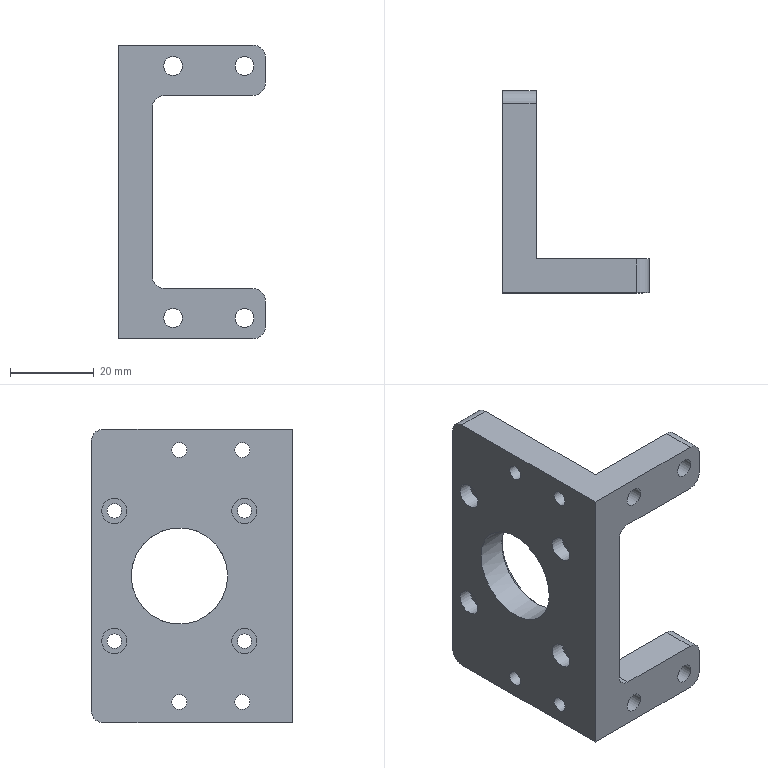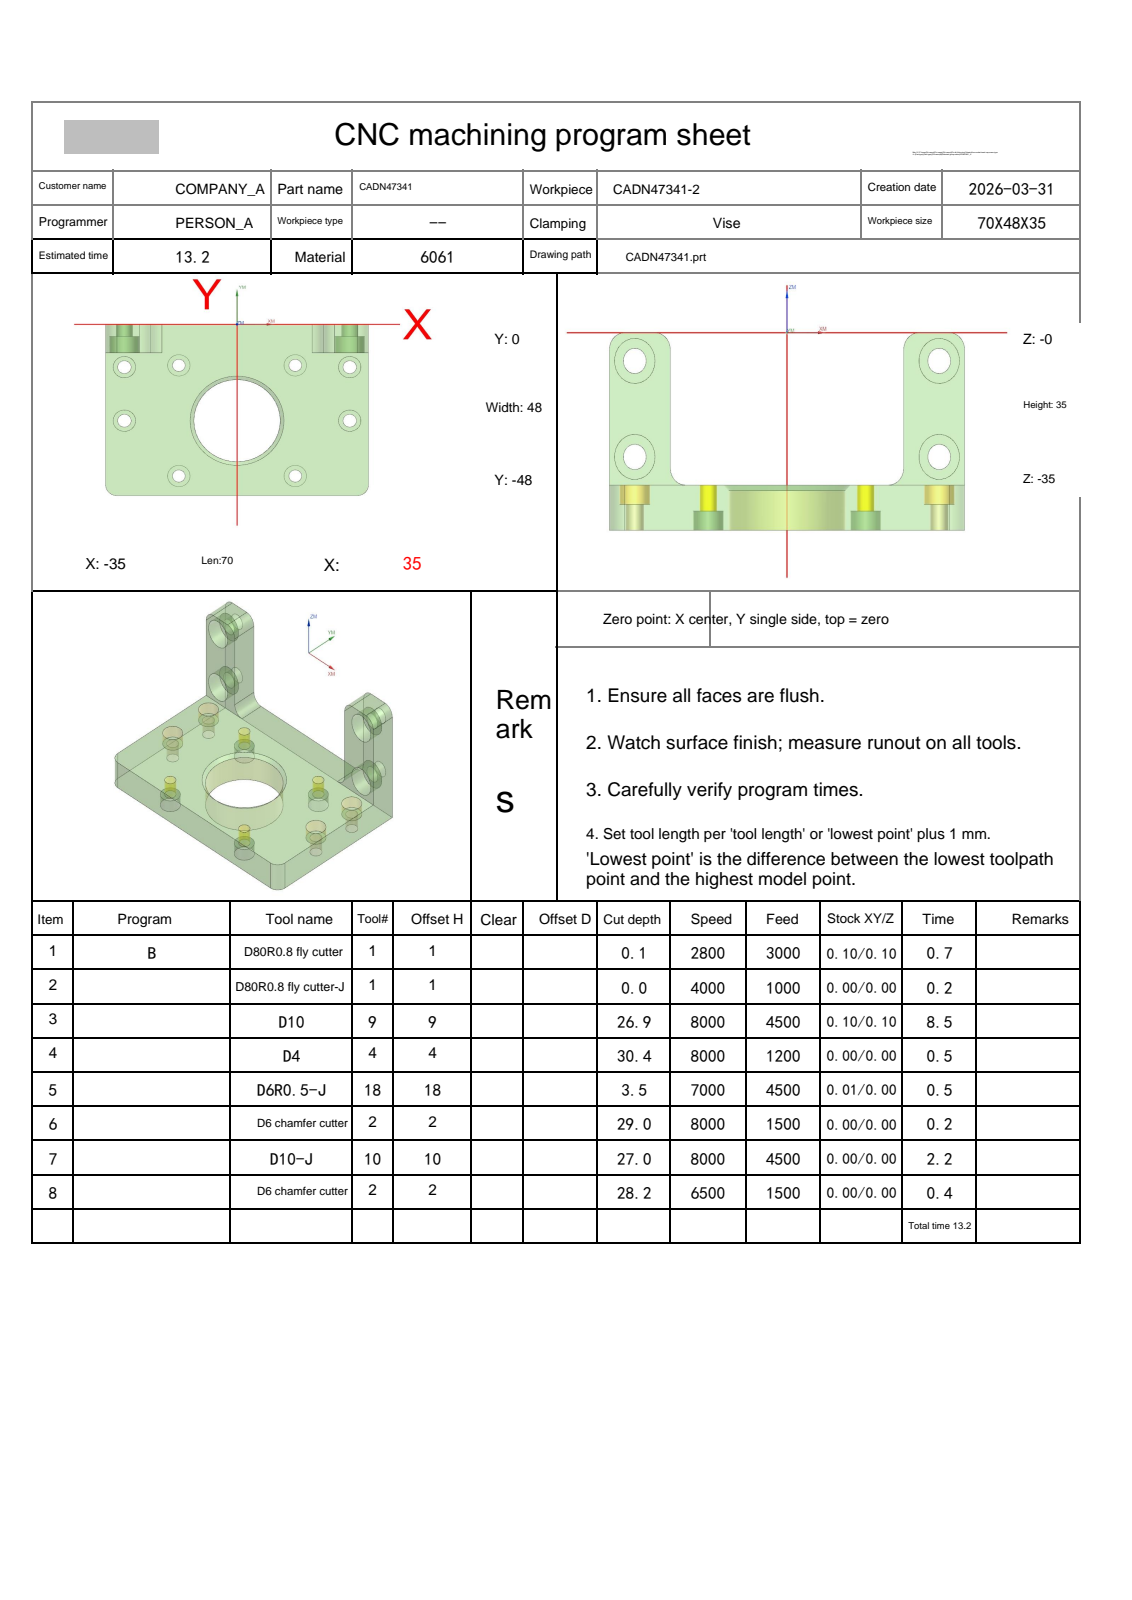NC program | NX | posted by the shop | part box 35 x 48 x 70 mm
Lines 9806 to 11022 of 13995:
N7 T10 M06
(D10-J  D=10. R=0. H=10 ce=0.40 di=0.00)
G00 G90 G54 X2. Y-55. M03 S7000
G43 H10 Z14.5
M08
Z-25.5
G01 Z-27. F1500.
Y-51.
G03 X0.0 Y-49. I-2. J0.0
G01 X-32.001
G02 X-36. Y-45. I.001 J4.
G01 Y-14.397
G02 X-35.003 Y-13.4 I1. J-.003
G01 X-14.6
Y.003
G02 X-13.603 Y1. I1. J-.003
G01 X13.603
G02 X14.6 Y.003 I-.003 J-1.
G01 Y-13.4
X35.003
G02 X36. Y-14.397 I-.003 J-1.
G01 Y-45.
G02 X32. Y-49. I-4. J0.0
G01 X-2.086
G02 X-2.793 Y-48.707 I.001 J1.
G01 X-7.207 Y-44.293
G03 X-7.914 Y-44. I-.707 J-.707
G01 X-30.003
G02 X-31. Y-43.003 I.003 J1.
G01 Y-19.397
G02 X-30.003 Y-18.4 I1. J-.003
G01 X-14.6
G03 X-9.6 Y-13.4 I0.0 J5.
G01 Y-4.997
G02 X-8.603 Y-4. I1. J-.003
G01 X8.603
G02 X9.6 Y-4.997 I-.003 J-1.
G01 Y-13.4
G03 X14.6 Y-18.4 I5. J0.0
G01 X30.003
G02 X31. Y-19.397 I-.003 J-1.
G01 Y-43.003
G02 X30.003 Y-44. I-1. J.003
G01 X-2.086
G02 X-2.793 Y-43.707 I0.0 J1.
G01 X-7.207 Y-39.293
G03 X-7.914 Y-39. I-.707 J-.707
G01 X-25.003
G02 X-26. Y-38.003 I.003 J1.
G01 Y-24.397
G02 X-25.003 Y-23.4 I1. J-.003
G01 X-14.6
G03 X-4.6 Y-13.4 I0.0 J10.
G01 Y-9.997
G02 X-3.603 Y-9. I1. J-.003
G01 X3.603
G02 X4.6 Y-9.997 I-.003 J-1.
G01 Y-13.4
G03 X14.6 Y-23.4 I10. J0.0
G01 X25.003
G02 X26. Y-24.397 I-.003 J-1.
G01 Y-38.003
G02 X25.003 Y-39. I-1. J.003
G01 X-2.086
G02 X-2.793 Y-38.707 I0.0 J1.
G01 X-7.207 Y-34.293
G03 X-7.914 Y-34. I-.707 J-.707
G01 X-20.003
G02 X-21. Y-33.003 I.003 J1.
G01 Y-29.397
G02 X-20.003 Y-28.4 I1. J-.003
G01 X-14.6
G03 X-.911 Y-19.533 I0.0 J15.
G02 X0.0 Y-18.945 I.911 J-.412
X.911 Y-19.533 I0.0 J-1.
G03 X14.6 Y-28.4 I13.689 J6.133
G01 X20.003
G02 X21. Y-29.397 I-.003 J-1.
G01 Y-33.003
G02 X20.003 Y-34. I-1. J.003
G01 X-1.511
G02 X-2.211 Y-33.3 I0.0 J.7
X-2.171 Y-33.067 I.7 J0.0
G01 X-1.072 Y-29.948
G03 X-.888 Y-28.876 I-3.044 J1.073
X-.923 Y-28.403 I-3.227 J0.0
G01 X-.931 Y-28.3
G02 X-.719 Y-27.798 I.7 J0.0
G03 X-.492 Y-27.576 I-13.881 J14.398
G02 X0.0 Y-27.374 I.492 J-.498
X.492 Y-27.576 I0.0 J-.7
G03 X.719 Y-27.798 I14.108 J14.176
G02 X.931 Y-28.3 I-.488 J-.502
X.233 Y-29. I-.7 J0.0
G01 X-.233
G02 X-.68 Y-28.837 I.003 J.7
X-.931 Y-28.3 I.449 J.537
X-.826 Y-27.931 I.7 J0.0
G03 X-.526 Y-26.878 I-1.7 J1.053
X-1.473 Y-25.178 I-2. J0.0
G01 Z-25.5
G00 Z14.5
G00 G90 X-13.5 Y-14.7 M03 S8000
Z14.5
Z-12.
G01 Z-13.5 F1000.
G41 D10
Y-14.5
G03 X-15. Y-13. I-1.5 J0.0
G01 X-40.
G03 X-41.5 Y-14.5 I0.0 J-1.5
G01 G40 Y-14.7
Z-12.
G00 X-13.5
Z-25.5
G01 Z-27.
G41 D10
Y-14.5
G03 X-15. Y-13. I-1.5 J0.0
G01 X-40.003
G03 X-41.5 Y-14.405 I0.0 J-1.5
G01 G40 X-41.513 Y-14.605
Z-25.5
G00 Z3.
X41.5 Y-14.7
Z-12.
G01 Z-13.5
G41 D10
Y-14.5
G03 X40. Y-13. I-1.5 J0.0
G01 X15.
G03 X13.5 Y-14.5 I0.0 J-1.5
G01 G40 Y-14.7
Z-12.
G00 X41.5
Z-25.5
G01 Z-27.
G41 D10
Y-14.5
G03 X40. Y-13. I-1.5 J0.0
G01 X14.997
G03 X13.5 Y-14.405 I0.0 J-1.5
G01 G40 X13.487 Y-14.605
Z-25.5
G00 Z14.5
G00 G90 X42. Y-15.199 M03 S8000
Z14.5
Z-26.
G01 Z-27. F1000.
G41 D10
Y-14.999
G03 X40. Y-13. I-2. J-.001
G01 X15.
Y5.
G03 X13.001 Y7. I-2. J0.0
G01 G40 X12.801
Z-26.
G00 X-12.801
G01 Z-27.
G41 D10
X-13.001
G03 X-15. Y5. I.001 J-2.
G01 Y-13.
X-40.
G03 X-42. Y-14.999 I0.0 J-2.
G01 G40 Y-15.199
Z-26.
G00 Z14.5
G00 G90 X16.3 Y-14.5 M03 S8000
Z14.5
Z-12.
G01 Z-13.5 F1000.
G41 D10
X16.5
G03 X18. Y-13. I0.0 J1.5
G01 Y5.
G03 X16.5 Y6.5 I-1.5 J0.0
G01 G40 X16.3
Z-12.
G00 X16.395 Y-14.513
Z-22.5
G01 Z-24.
G41 D10
X16.595 Y-14.5
G03 X18. Y-13.003 I-.095 J1.497
G01 Y5.003
G03 X16.595 Y6.5 I-1.5 J0.0
G01 G40 X16.395 Y6.513
Z-22.5
G00 Z0.0
X-16.3 Y6.5
Z-12.
G01 Z-13.5
G41 D10
X-16.5
G03 X-18. Y5. I0.0 J-1.5
G01 Y-13.
G03 X-16.5 Y-14.5 I1.5 J0.0
G01 G40 X-16.3
Z-12.
G00 X-16.301 Y6.5
Z-22.5
G01 Z-24.
G41 D10
X-16.501
G03 X-18. Y5. I.001 J-1.5
G01 Y-13.003
G03 X-16.595 Y-14.5 I1.5 J0.0
G01 G40 X-16.395 Y-14.513
Z-22.5
G00 Z14.5
G00 G90 X17.99 Y-17.768 M03 S7000
Z14.5
Z-23.515
G01 Z-24.015 F4500.
X17.989 Y-8.955
X17.988 Y.973
X17.99 Y1.027
X17.988 Z-24.03
Y-8.956
X17.986 Y-8.958 Z-24.045
X17.987 Y-8.058
Y0.0
Y1.028
X17.985 Y1.029 Z-24.06
X17.984 Y.973
X17.986 Y.081
X17.989 Y0.0
Y-7.939
X17.986 Y-8.058
X17.985 Y-8.96
X17.983 Y-8.961 Z-24.075
X17.985 Y-8.058
X17.989 Y-7.939
Y0.0
X17.985 Y.081
X17.983 Y1.03
X17.982 Y1.031 Z-24.09
X17.984 Y.081
X17.989 Y0.0
Y-7.946
X17.984 Y-8.058
X17.982 Y-8.963
X17.98 Y-8.964 Z-24.105
X17.979 Y-8.837
X17.985 Y-7.961
X17.988 Y-7.946
Y0.0
X17.983 Y.081
X17.979 Y.973
X17.98 Y1.031
X17.979 Y1.032 Z-24.12
X17.977 Y.973
X17.982 Y.081
X17.988 Y0.0
Y-7.939
X17.983 Y-7.989
X17.978 Y-8.837
X17.979 Y-8.966
X17.977 Y-8.968 Z-24.135
X17.983 Y-7.961
X17.987 Y-7.939
Y0.0
X17.981 Y.081
X17.976 Y.973
X17.977 Y1.033
X17.976 Y1.034 Z-24.15
X17.98 Y.081
X17.986 Y0.0
Y-7.939
X17.982 Y-7.961
X17.976 Y-8.969
X17.974 Y-8.971 Z-24.165
X17.981 Y-7.961
X17.985 Y-7.939
Y0.0
X17.979 Y.081
X17.974 Y1.034
X17.973 Y1.035 Z-24.18
X17.978 Y.081
X17.985 Y0.0
Y-7.939
X17.98 Y-7.961
X17.973 Y-8.972
X17.971 Y-8.974 Z-24.195
X17.979 Y-7.961
X17.984 Y-7.939
Y0.0
X17.977 Y.081
X17.971 Y1.036
X17.969 Y1.037 Z-24.21
X17.976 Y.081
X17.983 Y0.0
Y-7.939
X17.977 Y-7.989
X17.97 Y-8.976
X17.968 Y-8.977 Z-24.225
X17.973 Y-8.002
X17.982 Y-7.939
Y0.0
X17.975 Y.081
X17.968 Y1.037
X17.966 Y1.038 Z-24.24
X17.965 Y.973
X17.974 Y.081
X17.98 Y0.0
Y-7.939
X17.976 Y-7.961
X17.974 Y-8.058
X17.966 Y-8.979
X17.965 Y-8.98 Z-24.255
X17.964 Y-8.837
X17.972 Y-8.058
X17.975 Y-7.961
X17.979 Y-7.939
Y0.0
X17.973 Y.081
X17.963 Y.973
X17.965 Y1.039
X17.963 Y1.04 Z-24.269
X17.962 Y.973
X17.972 Y.081
X17.978 Y0.0
Y-7.939
X17.974 Y-7.961
X17.971 Y-8.058
X17.962 Y-8.837
X17.963 Y-8.982
X17.962 Y-8.984 Z-24.284
X17.961 Y-8.837
X17.971 Y-7.996
X17.976 Y-7.939
Y0.0
X17.971 Y.081
X17.96 Y.973
X17.962 Y1.041
X17.96 Z-24.299
G03 X17.957 Y.748 I15.859 J-.293
X17.975 Y0.0 I15.862 J0.0
G01 Y-7.939
X17.97 Y-7.995
X17.959 Y-8.837
X17.96 Y-8.985
X17.959 Y-8.987 Z-24.314
G02 X17.956 Y-8.697 I17.003 J.29
X17.968 Y-8.058 I17.006 J0.0
G01 X17.964 Y-8.002
X17.981 Y-7.972
X17.973 Y-7.939
Y0.0
G02 X17.956 Y.751 I16.031 J.751
X17.959 Y1.042 I16.049 J0.0
G01 X17.957 Y1.043 Z-24.329
G03 X17.954 Y.753 I16.196 J-.29
X17.972 Y0.0 I16.198 J0.0
G01 Y-7.939
X17.955 Y-7.998
X17.967 Y-8.057
G03 X17.955 Y-8.7 I16.404 J-.642
X17.957 Y-8.988 I16.417 J0.0
G01 X17.956 Y-8.99 Z-24.344
X17.954 Y-8.837
X17.966 Y-7.983
X17.97 Y-7.939
Y0.0
G02 X17.953 Y.752 I16.244 J.752
X17.955 Y1.044 I16.262 J0.0
G01 X17.954 Z-24.359
X17.952 Y.973
X17.964 Y.081
X17.968 Y0.0
Y-7.892
X17.966 Y-7.939
X17.965 Y-7.988
X17.953 Y-8.837
X17.954 Y-8.992
X17.953 Y-8.993 Z-24.374
X17.951 Y-8.837
X17.963 Y-7.96
X17.967 Y-7.939
Y0.0
X17.962 Y.081
X17.951 Y.973
X17.952 Y1.045
X17.951 Y1.046 Z-24.389
X17.949 Y.973
X17.96 Y.081
X17.965 Y0.0
Y-7.939
X17.961 Y-7.96
X17.95 Y-8.837
X17.951 Y-8.995
X17.949 Y-8.996 Z-24.404
X17.955 Y-8.001
X17.963 Y-7.939
Y0.0
X17.958 Y.081
X17.948 Y.973
X17.949 Y1.047
X17.947 Z-24.418
X17.956 Y.081
X17.961 Y0.0
Y-7.939
X17.954 Y-8.001
X17.948 Y-8.998
X17.945 Y-8.999 Z-24.433
X17.956 Y-7.96
X17.959 Y-7.939
Y0.0
X17.954 Y.081
X17.943 Y.973
X17.945 Y1.048
X17.942 Y1.049 Z-24.448
X17.94 Y.973
X17.952 Y.081
X17.956 Y0.0
Y-7.939
X17.951 Y-8.001
X17.943 Y-9.001
X17.94 Y-9.002 Z-24.463
X17.938 Y-8.837
X17.951 Y-7.988
X17.954 Y-7.96
Y0.0
X17.95 Y.081
X17.937 Y.973
X17.939 Y1.049
X17.937 Y1.05 Z-24.478
G03 X17.934 Y.762 I16.4 J-.289
X17.952 Y0.0 I16.403 J0.0
G01 Y-7.975
X17.949 Y-7.988
X17.936 Y-8.837
X17.937 Y-9.004
X17.934 Y-9.006 Z-24.492
X17.933 Y-8.837
X17.947 Y-8.001
X17.949 Y-7.988
Y0.0
G02 X17.931 Y.759 I15.925 J.759
X17.934 Y1.051 I15.943 J0.0
G01 X17.931 Y1.052 Z-24.507
G03 X17.928 Y.755 I15.491 J-.297
X17.947 Y0.0 I15.494 J0.0
G01 Y-8.
X17.943 Y-8.057
X17.93 Y-8.837
X17.932 Y-9.007
X17.929 Y-9.009 Z-24.522
X17.927 Y-8.837
X17.94 Y-8.057
X17.944 Y-8.
Y0.0
G02 X17.926 Y.752 I15.13 J.752
X17.929 Y1.053 I15.149 J0.0
G01 X17.926 Z-24.537
G03 X17.923 Y.748 I14.891 J-.305
X17.942 Y0.0 I14.894 J0.0
G01 Y-8.
X17.936 Y-8.057
X17.925 Y-8.837
X17.926 Y-9.01
X17.923 Y-9.012 Z-24.551
X17.922 Y-8.837
X17.933 Y-8.057
X17.939 Y-8.
Y0.0
X17.933 Y.081
X17.921 Y.973
X17.923 Y1.054
X17.921 Y1.055 Z-24.566
X17.919 Y.973
X17.93 Y.081
X17.936 Y0.0
Y-8.
X17.93 Y-8.056
X17.919 Y-8.837
X17.921 Y-9.014
X17.918 Y-9.015 Z-24.581
X17.916 Y-8.837
X17.927 Y-8.056
X17.933 Y-8.
Y0.0
X17.927 Y.081
X17.916 Y.973
X17.918 Y1.056
X17.915 Y1.057 Z-24.596
X17.913 Y.973
X17.923 Y.081
X17.93 Y0.0
Y-8.
X17.924 Y-8.056
X17.914 Y-8.837
X17.915 Y-9.017
X17.912 Y-9.018 Z-24.61
X17.921 Y-8.056
X17.927 Y-8.
Y0.0
X17.92 Y.081
X17.911 Y.973
X17.913 Y1.057
X17.91 Y1.058 Z-24.625
X17.908 Y.973
X17.917 Y.081
X17.924 Y0.0
Y-8.
X17.918 Y-8.056
X17.91 Y-9.02
X17.907 Y-9.022 Z-24.64
X17.915 Y-8.056
X17.921 Y-8.
Y0.0
X17.914 Y.081
X17.905 Y.973
X17.907 Y1.059
X17.904 Y1.06 Z-24.654
X17.902 Y.973
X17.911 Y.081
X17.918 Y0.0
Y-8.
X17.912 Y-8.056
X17.904 Y-9.023
X17.9 Y-9.025 Z-24.669
G02 X17.897 Y-8.747 I16.4 J.278
X17.914 Y-8. I16.402 J0.0
G01 Y0.0
X17.908 Y.081
X17.898 Y.973
X17.9 Y1.06
X17.896 Y1.061 Z-24.683
G03 X17.892 Y.728 I14.19 J-.333
X17.911 Y0.0 I14.194 J0.0
G01 Y-8.
X17.906 Y-8.056
X17.894 Y-8.837
X17.896 Y-9.026
X17.892 Y-9.028 Z-24.698
X17.89 Y-8.837
X17.903 Y-8.056
X17.908 Y-8.
Y0.0
G02 X17.888 Y.73 I13.763 J.73
X17.892 Y1.062 I13.783 J0.0
G01 X17.888 Y1.063 Z-24.713
G03 X17.884 Y.731 I13.342 J-.332
X17.904 Y0.0 I13.346 J0.0
G01 Y-8.
X17.898 Y-8.056
X17.886 Y-8.837
X17.888 Y-9.029
X17.884 Y-9.031 Z-24.727
X17.882 Y-8.837
X17.894 Y-8.055
X17.901 Y-8.
Y0.0
G02 X17.88 Y.731 I12.974 J.731
X17.884 Y1.063 I12.994 J0.0
G01 X17.88 Y1.064 Z-24.742
G03 X17.876 Y.731 I12.711 J-.333
X17.897 Y0.0 I12.716 J0.0
G01 Y-7.987
X17.892 Y-8.
X17.878 Y-8.837
X17.88 Y-9.032
X17.876 Y-9.034 Z-24.756
X17.874 Y-8.837
X17.888 Y-8.
X17.893 Y-7.986
Y0.0
G02 X17.872 Y.732 I12.48 J.732
X17.876 Y1.065 I12.502 J0.0
G01 X17.872 Y1.066 Z-24.771
G03 X17.868 Y.732 I12.342 J-.334
X17.889 Y0.0 I12.346 J0.0
G01 Y-7.986
X17.884 Y-7.999
X17.87 Y-8.837
X17.872 Y-9.036
X17.867 Y-9.037 Z-24.785
G02 X17.865 Y-8.75 I20.319 J.287
X17.877 Y-8.055 I20.321 J0.0
G01 X17.885 Y-7.986
Y0.0
G02 X17.864 Y.732 I12.223 J.732
X17.868 Y1.067 I12.245 J0.0
G01 X17.864 Y1.068 Z-24.8
G03 X17.859 Y.732 I12.191 J-.336
X17.881 Y0.0 I12.196 J0.0
G01 Y-7.986
X17.873 Y-8.055
G03 X17.861 Y-8.75 I20.656 J-.695
X17.863 Y-9.039 I20.668 J0.0
G01 X17.859 Y-9.04 Z-24.814
G02 X17.857 Y-8.75 I21.024 J.291
X17.869 Y-8.055 I21.026 J0.0
G01 X17.877 Y-7.986
Y0.0
G02 X17.855 Y.732 I12.174 J.732
X17.86 Y1.068 I12.196 J0.0
G01 X17.856 Y1.069 Z-24.828
X17.854 Y.973
X17.864 Y.081
X17.873 Y0.0
Y-7.986
X17.865 Y-8.055
G03 X17.853 Y-8.75 I21.383 J-.695
X17.855 Y-9.042 I21.394 J0.0
G01 X17.851 Y-9.043 Z-24.843
G02 X17.849 Y-8.75 I21.771 J.294
X17.861 Y-8.055 I21.773 J0.0
G01 X17.869 Y-7.986
Y0.0
X17.86 Y.081
X17.85 Y.973
X17.852 Y1.07
X17.848 Y1.071 Z-24.857
X17.846 Y.973
X17.856 Y.081
X17.865 Y0.0
Y-7.986
X17.856 Y-8.054
G03 X17.845 Y-8.75 I22.153 J-.695
X17.847 Y-9.045 I22.164 J0.0
G01 X17.843 Y-9.046 Z-24.872
X17.842 Y-8.837
X17.855 Y-7.999
X17.861 Y-7.986
Y0.0
X17.851 Y.081
X17.842 Y.973
X17.844 Y1.072
X17.84 Z-24.886
X17.838 Y.973
X17.847 Y.081
X17.856 Y0.0
Y-7.985
X17.848 Y-8.054
X17.839 Y-9.048
X17.836 Y-9.05 Z-24.9
X17.844 Y-8.054
X17.852 Y-7.998
Y0.0
X17.843 Y.081
X17.834 Y.973
X17.836 Y1.073
X17.832 Y1.074 Z-24.915
X17.83 Y.973
X17.839 Y.081
X17.847 Y0.0
Y-7.998
X17.84 Y-8.054
X17.832 Y-9.051
X17.828 Y-9.053 Z-24.929
X17.836 Y-8.054
X17.843 Y-7.998
Y0.0
X17.835 Y.081
X17.826 Y.973
X17.828 Y1.075
X17.824 Y1.076 Z-24.943
X17.822 Y.973
X17.831 Y.081
X17.838 Y0.0
Y-8.
X17.831 Y-8.054
X17.824 Y-9.054
X17.82 Y-9.056 Z-24.957
X17.827 Y-8.054
X17.833 Y-8.
Y0.0
X17.827 Y.081
X17.818 Y.973
X17.82 Y1.076
X17.815 Y1.077 Z-24.971
X17.813 Y.973
X17.823 Y.081
X17.828 Y0.0
Y-8.
X17.823 Y-8.054
X17.815 Y-9.057
X17.809 Y-9.059 Z-24.986
G02 X17.806 Y-8.753 I16.666 J.306
X17.823 Y-8. I16.669 J0.0
G01 Y0.0
G02 X17.806 Y.724 I14.843 J.724
X17.81 Y1.078 I14.861 J0.0
G01 X17.805 Z-25.
G03 X17.8 Y.726 I14.471 J-.352
X17.819 Y0.0 I14.475 J0.0
G01 Y-8.
G03 X17.801 Y-8.754 I16.127 J-.754
X17.804 Y-9.06 I16.144 J0.0
G01 X17.798 Y-9.062 Z-25.014
G02 X17.795 Y-8.754 I15.629 J.308
X17.814 Y-8. I15.632 J0.0
G01 Y0.0
G02 X17.795 Y.727 I14.08 J.727
X17.799 Y1.079 I14.098 J0.0
G01 X17.794 Y1.08 Z-25.028
G03 X17.789 Y.728 I13.802 J-.352
X17.808 Y0.0 I13.806 J0.0
G01 Y-8.
G03 X17.79 Y-8.754 I15.22 J-.754
X17.793 Y-9.063 I15.239 J0.0
G01 X17.787 Y-9.065 Z-25.042
G02 X17.784 Y-8.754 I14.943 J.311
X17.803 Y-8. I14.947 J0.0
G01 Y0.0
G02 X17.784 Y.729 I13.569 J.729
X17.788 Y1.081 I13.589 J0.0
G01 X17.783 Y1.082 Z-25.056
G03 X17.778 Y.729 I13.434 J-.352
X17.798 Y0.0 I13.439 J0.0
G01 Y-8.
G03 X17.779 Y-8.754 I14.726 J-.754
X17.782 Y-9.066 I14.745 J0.0
G01 X17.777 Y-9.068 Z-25.07
G02 X17.773 Y-8.754 I14.624 J.314
X17.793 Y-8. I14.627 J0.0
G01 Y0.0
G02 X17.773 Y.73 I13.333 J.73
X17.777 Y1.083 I13.353 J0.0
G01 X17.772 Z-25.084
G03 X17.767 Y.73 I13.322 J-.353
X17.787 Y0.0 I13.327 J0.0
G01 Y-8.
G03 X17.768 Y-8.754 I14.567 J-.754
X17.771 Y-9.069 I14.587 J0.0
G01 X17.766 Y-9.071 Z-25.098
G02 X17.762 Y-8.755 I14.619 J.316
X17.782 Y-8. I14.622 J0.0
G01 Y0.0
G02 X17.762 Y.73 I13.341 J.73
X17.767 Y1.084 I13.361 J0.0
G01 X17.761 Y1.085 Z-25.112
G03 X17.757 Y.73 I13.451 J-.355
X17.776 Y0.0 I13.455 J0.0
G01 Y-7.996
G03 X17.757 Y-8.755 I14.857 J-.758
X17.76 Y-9.072 I14.877 J0.0
G01 X17.755 Y-9.074 Z-25.126
G02 X17.752 Y-8.756 I14.923 J.318
X17.771 Y-8. I14.926 J0.0
G01 Y0.0
X17.763 Y.081
X17.753 Y.973
X17.756 Y1.086
X17.75 Y1.087 Z-25.14
X17.748 Y.973
X17.758 Y.081
X17.765 Y0.0
Y-8.
G03 X17.746 Y-8.756 I15.183 J-.756
X17.75 Y-9.075 I15.202 J0.0
G01 X17.744 Y-9.077 Z-25.153
G02 X17.741 Y-8.757 I15.567 J.32
X17.759 Y-8. I15.57 J0.0
G01 Y0.0
X17.752 Y.081
X17.743 Y.973
X17.745 Y1.087
X17.74 Y1.088 Z-25.167
X17.737 Y.973
X17.747 Y.081
X17.754 Y0.0
Y-8.
G03 X17.736 Y-8.757 I16.026 J-.757
X17.739 Y-9.078 I16.044 J0.0
G01 X17.734 Y-9.08 Z-25.181
G02 X17.73 Y-8.758 I16.637 J.322
X17.748 Y-8. I16.64 J0.0
G01 Y0.0
X17.741 Y.081
X17.732 Y.973
X17.734 Y1.089
X17.728 Y1.09 Z-25.195
G03 X17.724 Y.725 I14.539 J-.365
X17.742 Y0.0 I14.544 J0.0
G01 Y-8.
G03 X17.724 Y-8.759 I16.476 J-.759
X17.728 Y-9.081 I16.493 J0.0
G01 X17.721 Y-9.083 Z-25.209
G02 X17.718 Y-8.761 I16.057 J.322
X17.736 Y-8. I16.06 J0.0
G01 Y0.0
G02 X17.717 Y.726 I14.158 J.726
X17.722 Y1.091 I14.177 J0.0
G01 X17.715 Z-25.222
G03 X17.711 Y.727 I13.841 J-.364
X17.73 Y0.0 I13.846 J0.0
G01 Y-8.
G03 X17.711 Y-8.761 I15.587 J-.761
X17.714 Y-9.084 I15.605 J0.0
G01 X17.708 Y-9.086 Z-25.236
G02 X17.705 Y-8.762 I15.257 J.324
X17.724 Y-8. I15.26 J0.0
G01 Y0.0
G02 X17.704 Y.729 I13.574 J.729
X17.709 Y1.092 I13.593 J0.0
G01 X17.702 Y1.093 Z-25.25
G03 X17.698 Y.73 I13.407 J-.363
X17.717 Y0.0 I13.412 J0.0
G01 Y-8.
G03 X17.698 Y-8.763 I14.992 J-.763
X17.702 Y-9.087 I15.011 J0.0
G01 X17.695 Y-9.089 Z-25.263
G02 X17.692 Y-8.763 I14.845 J.326
X17.711 Y-8. I14.849 J0.0
G01 Y0.0
G02 X17.691 Y.731 I13.275 J.731
X17.696 Y1.094 I13.295 J0.0
G01 X17.69 Y1.095 Z-25.277
G03 X17.685 Y.732 I13.235 J-.363
X17.705 Y0.0 I13.24 J0.0
G01 Y-8.
G03 X17.685 Y-8.764 I14.747 J-.764
X17.689 Y-9.09 I14.767 J0.0
G01 X17.682 Y-9.092 Z-25.29
G02 X17.679 Y-8.765 I14.759 J.327
X17.698 Y-8. I14.762 J0.0
G01 Y0.0
G02 X17.678 Y.732 I13.224 J.732
X17.683 Y1.095 I13.245 J0.0
G01 X17.677 Y1.096 Z-25.304
X17.674 Y.973
X17.684 Y.081
X17.692 Y0.0
Y-8.
G03 X17.672 Y-8.765 I14.814 J-.765
X17.676 Y-9.093 I14.834 J0.0
G01 X17.669 Y-9.095 Z-25.317
G02 X17.666 Y-8.766 I14.98 J.329
X17.685 Y-8. I14.983 J0.0
G01 Y0.0
X17.677 Y.081
X17.668 Y.973
X17.67 Y1.097
X17.664 Y1.098 Z-25.331
X17.661 Y.973
X17.671 Y.081
X17.679 Y0.0
Y-8.
G03 X17.659 Y-8.767 I15.195 J-.767
X17.663 Y-9.096 I15.214 J0.0
G01 X17.657 Y-9.098 Z-25.344
G02 X17.653 Y-8.767 I15.505 J.331
X17.672 Y-8. I15.509 J0.0
G01 Y0.0
X17.664 Y.081
X17.655 Y.973
X17.658 Y1.099
X17.651 Z-25.357
X17.648 Y.973
X17.658 Y.081
X17.665 Y0.0
Y-8.
G03 X17.647 Y-8.768 I15.933 J-.768
X17.65 Y-9.099 I15.951 J0.0
G01 X17.644 Y-9.1 Z-25.371
G02 X17.64 Y-8.767 I16.105 J.333
X17.659 Y-8. I16.109 J0.0
G01 Y0.0
X17.651 Y.081
X17.642 Y.973
X17.644 Y1.1
X17.637 Z-25.384
G03 X17.632 Y.729 I13.663 J-.371
X17.652 Y0.0 I13.668 J0.0
G01 Y-8.
G03 X17.633 Y-8.768 I15.535 J-.768
X17.636 Y-9.1 I15.554 J0.0
G01 X17.629 Z-25.397
G02 X17.625 Y-8.773 I15.403 J.327
X17.645 Y-8. I15.406 J0.0
G01 Y0.0
G02 X17.625 Y.731 I13.274 J.731
X17.63 Y1.1 I13.294 J0.0
G01 X17.622 Z-25.41
G03 X17.617 Y.732 I13.006 J-.368
X17.638 Y0.0 I13.012 J0.0
G01 Y-8.
G03 X17.618 Y-8.774 I15.012 J-.774
X17.621 Y-9.1 I15.032 J0.0
G01 X17.614 Z-25.424
G02 X17.61 Y-8.774 I14.742 J.325
X17.631 Y-8. I14.745 J0.0
G01 Y0.0
G02 X17.61 Y.733 I12.776 J.733
X17.615 Y1.1 I12.797 J0.0
G01 X17.607 Z-25.437
G03 X17.602 Y.735 I12.638 J-.365
X17.624 Y0.0 I12.644 J0.0
G01 Y-8.
G03 X17.603 Y-8.775 I14.517 J-.775
X17.607 Y-9.1 I14.537 J0.0
G01 X17.599 Z-25.45
G02 X17.595 Y-8.775 I14.399 J.325
X17.616 Y-8. I14.402 J0.0
G01 Y0.0
G02 X17.595 Y.735 I12.527 J.735
X17.6 Y1.1 I12.548 J0.0
G01 X17.593 Z-25.463
G03 X17.587 Y.736 I12.503 J-.363
X17.609 Y0.0 I12.508 J0.0
G01 Y-8.
G03 X17.588 Y-8.776 I14.315 J-.776
X17.592 Y-9.1 I14.336 J0.0
G01 X17.584 Z-25.476
G02 X17.581 Y-8.776 I14.332 J.324
X17.602 Y-8. I14.336 J0.0
G01 Y0.0
X17.593 Y.081
X17.582 Y.973
X17.585 Y1.1
X17.578 Y1.099 Z-25.489
X17.575 Y.973
X17.585 Y.081
X17.594 Y0.0
Y-8.
G03 X17.573 Y-8.776 I14.382 J-.776
X17.577 Y-9.1 I14.403 J0.0
G01 X17.57 Z-25.502
G02 X17.566 Y-8.776 I14.535 J.324
X17.587 Y-8. I14.538 J0.0
G01 Y0.0
X17.578 Y.081
X17.568 Y.973
X17.571 Y1.099
X17.563 Z-25.515
X17.561 Y.973
X17.57 Y.081
X17.579 Y0.0
Y-8.
G03 X17.559 Y-8.776 I14.726 J-.776
X17.563 Y-9.1 I14.746 J0.0
G01 X17.555 Z-25.528
G02 X17.552 Y-8.776 I15.03 J.324
X17.572 Y-8. I15.033 J0.0
G01 Y0.0
X17.563 Y.081
X17.553 Y.973
X17.556 Y1.099
X17.549 Z-25.541
X17.546 Y.973
X17.556 Y.081
X17.564 Y0.0
Y-8.
G03 X17.545 Y-8.776 I15.388 J-.776
X17.548 Y-9.1 I15.408 J0.0
G01 X17.541 Z-25.553
G02 X17.537 Y-8.776 I15.879 J.324
X17.556 Y-8. I15.883 J0.0
G01 Y0.0
X17.548 Y.081
X17.539 Y.973
X17.542 Y1.099
X17.534 Z-25.566
X17.532 Y.973
X17.541 Y.081
X17.549 Y0.0
Y-8.
G03 X17.53 Y-8.776 I16.354 J-.776
X17.533 Y-9.1 I16.372 J0.0
G01 X17.525 Z-25.579
G02 X17.522 Y-8.774 I15.865 J.326
X17.541 Y-8. I15.869 J0.0
G01 Y0.0
G02 X17.521 Y.732 I13.715 J.732
X17.526 Y1.099 I13.734 J0.0
G01 X17.518 Z-25.592
G03 X17.513 Y.733 I13.458 J-.366
X17.533 Y0.0 I13.463 J0.0
G01 Y-8.
G03 X17.514 Y-8.775 I15.483 J-.775
X17.517 Y-9.1 I15.503 J0.0
G01 X17.509 Z-25.604
G02 X17.505 Y-8.775 I15.228 J.325
X17.525 Y-8. I15.231 J0.0
G01 Y0.0
G02 X17.505 Y.735 I13.24 J.735
X17.51 Y1.099 I13.261 J0.0
G01 X17.501 Z-25.617
G03 X17.496 Y.736 I13.12 J-.363
X17.517 Y0.0 I13.125 J0.0
G01 Y-8.
G03 X17.497 Y-8.776 I15.024 J-.776
X17.5 Y-9.1 I15.044 J0.0
G01 X17.492 Z-25.63
G02 X17.489 Y-8.776 I14.933 J.324
X17.509 Y-8. I14.937 J0.0
G01 Y0.0
G02 X17.488 Y.737 I13.033 J.737
X17.493 Y1.099 I13.053 J0.0
G01 X17.485 Z-25.642
G03 X17.48 Y.737 I13.038 J-.362
X17.501 Y0.0 I13.043 J0.0
G01 Y-8.
G03 X17.48 Y-8.776 I14.885 J-.776
X17.484 Y-9.1 I14.905 J0.0
G01 X17.476 Z-25.655
G02 X17.472 Y-8.776 I14.945 J.323
X17.492 Y-8. I14.949 J0.0
G01 Y0.0
G02 X17.472 Y.738 I13.073 J.738
X17.477 Y1.099 I13.094 J0.0
G01 X17.469 Z-25.667
X17.466 Y.973
X17.476 Y.081
X17.484 Y0.0
Y-8.
G03 X17.464 Y-8.776 I15.049 J-.776
X17.468 Y-9.1 I15.069 J0.0
G01 X17.46 Z-25.679
G02 X17.456 Y-8.777 I15.265 J.323
X17.476 Y-8. I15.268 J0.0
G01 Y0.0
X17.468 Y.081
X17.458 Y.973
X17.46 Y1.099
X17.452 Z-25.692
X17.45 Y.973
X17.459 Y.081
X17.467 Y0.0
Y-8.
G03 X17.448 Y-8.777 I15.535 J-.777
X17.451 Y-9.1 I15.554 J0.0
G01 X17.443 Z-25.704
G02 X17.44 Y-8.776 I15.933 J.323
X17.459 Y-8. I15.936 J0.0
G01 Y0.0
X17.451 Y.081
X17.442 Y.973
X17.444 Y1.099
X17.436 Z-25.716
X17.434 Y.973
X17.443 Y.081
X17.45 Y0.0
Y-8.
G03 X17.432 Y-8.776 I16.409 J-.776
X17.435 Y-9.1 I16.427 J0.0
G01 X17.427 Z-25.729
G02 X17.424 Y-8.776 I17.044 J.324
X17.442 Y-8. I17.047 J0.0
G01 Y0.0
X17.435 Y.081
X17.426 Y.973
X17.428 Y1.099
X17.419 Z-25.741
G03 X17.415 Y.734 I14.581 J-.365
X17.433 Y0.0 I14.586 J0.0
G01 Y-8.
G03 X17.416 Y-8.773 I16.868 J-.773
X17.419 Y-9.1 I16.885 J0.0
G01 X17.409 Z-25.753
G02 X17.405 Y-8.774 I15.674 J.325
X17.425 Y-8. I15.678 J0.0
G01 Y0.0
G02 X17.405 Y.733 I13.592 J.733
X17.41 Y1.099 I13.612 J0.0
G01 X17.4 Z-25.765
G03 X17.395 Y.735 I12.834 J-.364
X17.416 Y0.0 I12.84 J0.0
G01 Y-8.
G03 X17.395 Y-8.775 I14.689 J-.775
X17.399 Y-9.1 I14.71 J0.0
G01 X17.389 Z-25.777
G02 X17.385 Y-8.776 I13.921 J.323
X17.407 Y-8. I13.925 J0.0
G01 Y0.0
G02 X17.385 Y.738 I12.186 J.738
X17.39 Y1.099 I12.208 J0.0
G01 X17.38 Z-25.789
G03 X17.375 Y.74 I11.682 J-.36
X17.398 Y0.0 I11.688 J0.0
G01 Y-8.
G03 X17.375 Y-8.777 I13.26 J-.777
X17.379 Y-9.1 I13.283 J0.0
G01 X17.369 Z-25.801
G02 X17.365 Y-8.778 I12.752 J.322
X17.389 Y-8. I12.756 J0.0
G01 Y0.0
G02 X17.365 Y.741 I11.235 J.741
X17.37 Y1.099 I11.259 J0.0
G01 X17.361 Z-25.813
G03 X17.355 Y.743 I10.901 J-.357
X17.38 Y0.0 I10.907 J0.0
G01 Y-8.
G03 X17.356 Y-8.778 I12.302 J-.778
X17.36 Y-9.1 I12.326 J0.0
G01 X17.35 Z-25.825
G02 X17.346 Y-8.778 I11.957 J.321
X17.371 Y-8. I11.961 J0.0
G01 Y0.0
G02 X17.345 Y.744 I10.593 J.744
X17.351 Y1.099 I10.619 J0.0
G01 X17.341 Z-25.837
G03 X17.335 Y.745 I10.382 J-.355
X17.362 Y0.0 I10.388 J0.0
G01 Y-8.
G03 X17.336 Y-8.779 I11.685 J-.779
X17.34 Y-9.1 I11.711 J0.0
G01 X17.331 Z-25.849
G02 X17.326 Y-8.779 I11.461 J.321
X17.353 Y-8. I11.465 J0.0
G01 Y0.0
G02 X17.326 Y.745 I10.18 J.745
X17.332 Y1.099 I10.207 J0.0
G01 X17.322 Z-25.86
G03 X17.316 Y.746 I10.065 J-.353
X17.344 Y0.0 I10.071 J0.0
G01 Y-8.
G03 X17.317 Y-8.78 I11.275 J-.78
X17.321 Y-9.1 I11.302 J0.0
G01 X17.312 Z-25.872
G02 X17.307 Y-8.78 I11.18 J.32
X17.334 Y-8. I11.184 J0.0
G01 Y0.0
G02 X17.306 Y.747 I9.959 J.747
X17.313 Y1.099 I9.987 J0.0
G01 X17.303 Y1.1 Z-25.884
G03 X17.297 Y.747 I9.916 J-.352
X17.325 Y0.0 I9.922 J0.0
G01 Y-8.
G03 X17.298 Y-8.78 I11.086 J-.78
X17.302 Y-9.1 I11.113 J0.0
G01 X17.293 Z-25.895
G02 X17.288 Y-8.78 I11.083 J.32
X17.316 Y-8. I11.088 J0.0
G01 Y0.0
G02 X17.287 Y.747 I9.878 J.747
X17.294 Y1.1 I9.906 J0.0
G01 X17.284 Z-25.907
G03 X17.278 Y.748 I9.921 J-.352
X17.306 Y0.0 I9.928 J0.0
G01 Y-8.
G03 X17.279 Y-8.78 I11.08 J-.78
X17.283 Y-9.1 I11.107 J0.0
G01 X17.274 Z-25.918
G02 X17.269 Y-8.78 I11.166 J.32
X17.297 Y-8. I11.171 J0.0
G01 Y0.0
G02 X17.269 Y.748 I9.96 J.748
X17.275 Y1.1 I9.988 J0.0
G01 X17.265 Z-25.93
G03 X17.259 Y.748 I10.082 J-.352
X17.287 Y0.0 I10.088 J0.0
G01 Y-8.
G03 X17.26 Y-8.78 I11.254 J-.78
X17.265 Y-9.1 I11.281 J0.0
G01 X17.255 Z-25.941
G02 X17.251 Y-8.78 I11.437 J.32
X17.277 Y-8. I11.441 J0.0
G01 Y0.0
G02 X17.25 Y.748 I10.203 J.748
X17.256 Y1.1 I10.23 J0.0
G01 X17.247 Z-25.952
G03 X17.241 Y.747 I10.412 J-.352
X17.268 Y0.0 I10.418 J0.0
G01 Y-8.
G03 X17.242 Y-8.78 I11.628 J-.78
X17.246 Y-9.1 I11.654 J0.0
G01 X17.237 Z-25.964
G02 X17.232 Y-8.78 I11.908 J.32
X17.258 Y-8. I11.912 J0.0
G01 Y0.0
G02 X17.232 Y.747 I10.63 J.747
X17.238 Y1.1 I10.656 J0.0
G01 X17.228 Z-25.975
G03 X17.223 Y.747 I10.946 J-.353
X17.248 Y0.0 I10.952 J0.0
G01 Y-8.
G03 X17.223 Y-8.78 I12.25 J-.78
X17.228 Y-9.1 I12.275 J0.0
G01 X17.218 Z-25.986
G02 X17.214 Y-8.78 I12.708 J.32
X17.238 Y-8. I12.712 J0.0
G01 Y0.0
G02 X17.214 Y.746 I11.289 J.746
X17.219 Y1.1 I11.313 J0.0
G01 X17.21 Z-25.997
G03 X17.205 Y.745 I11.747 J-.355
X17.228 Y0.0 I11.752 J0.0
G01 Y-8.
G03 X17.205 Y-8.779 I13.17 J-.779
X17.209 Y-9.1 I13.193 J0.0
G01 X17.2 Z-26.008
G02 X17.197 Y-8.779 I13.81 J.321
X17.218 Y-8. I13.814 J0.0
G01 Y0.0
G02 X17.196 Y.744 I12.261 J.744
X17.201 Y1.1 I12.284 J0.0
G01 X17.193 Z-26.014
X17.191 Z-26.019
G03 X17.185 Y.739 I11.576 J-.361
X17.208 Y0.0 I11.581 J0.0
G01 Y-8.
G03 X17.185 Y-8.771 I12.807 J-.771
X17.19 Y-9.1 I12.83 J0.0
G01 X17.178 Z-26.03
G02 X17.174 Y-8.778 I12.543 J.322
X17.198 Y-8. I12.547 J0.0
G01 Y-.001
G02 X17.174 Y.741 I11.087 J.742
X17.179 Y1.1 I11.112 J0.0
G01 X17.168 Z-26.041
G03 X17.162 Y.743 I10.647 J-.357
X17.188 Y0.0 I10.653 J0.0
G01 Y-8.
G03 X17.163 Y-8.778 I11.973 J-.778
X17.167 Y-9.1 I11.998 J0.0
G01 X17.163 Z-26.047
X17.156 Z-26.052
G02 X17.152 Y-8.779 I11.554 J.321
X17.178 Y-8. I11.559 J0.0
G01 Y0.0
G02 X17.151 Y.744 I10.267 J.744
X17.157 Y1.1 I10.294 J0.0